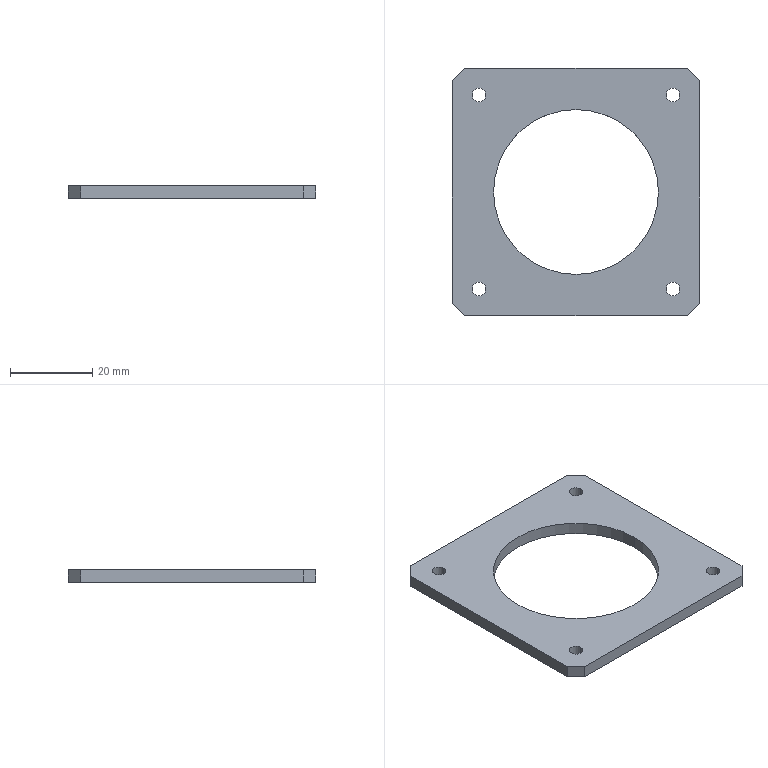Part | STEP file | PN_0043 | 1 solid | 20 faces | box 60 x 60 x 3 mm | volume 6873 mm3 | cylinder 10 | plane 10 | commonest cylinder face diameters 3.3 x8 40 x2